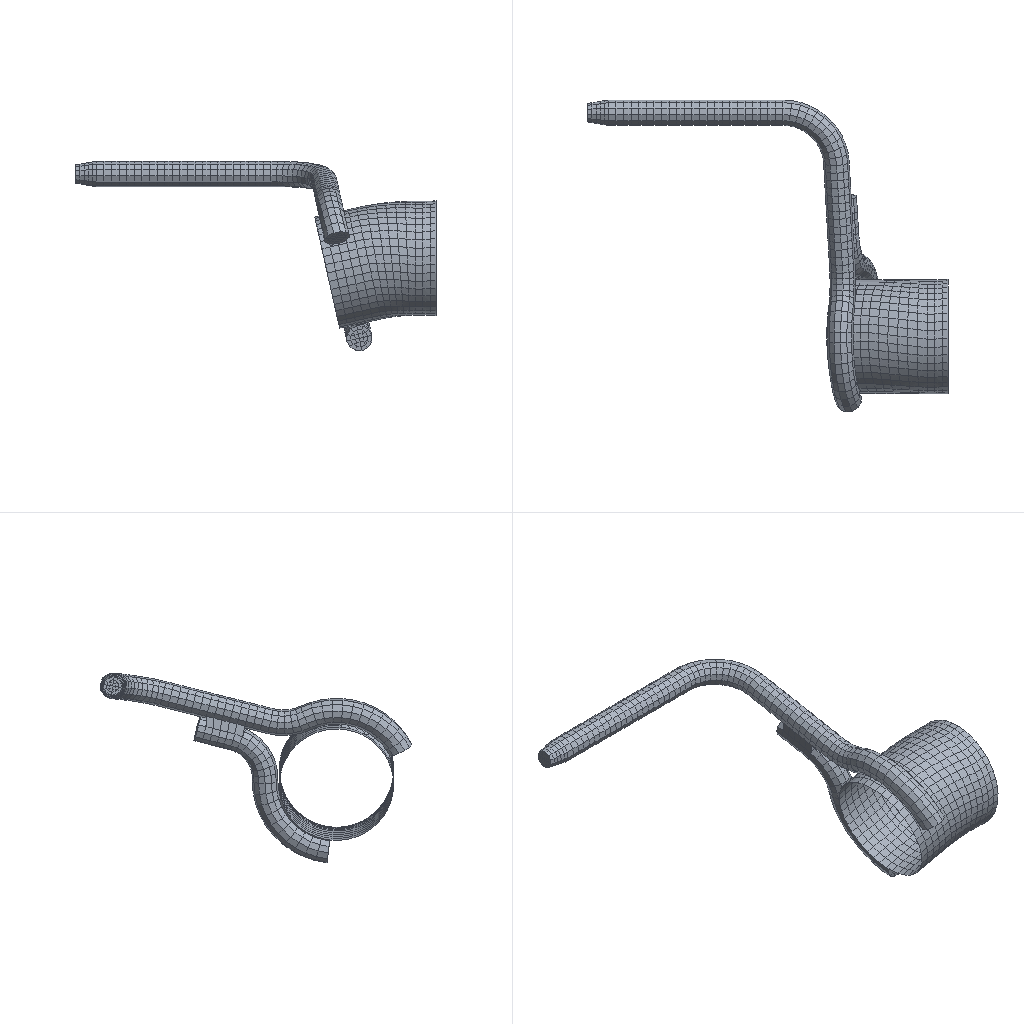Simulation study | nastran
Set-up summary:
category,name,step,type,value,unit,region
solver,nx_nastran
units,not stated in the deck,,not stated
analysis,deck,,modal,modal
analysis,solution,,SOL,103
load_step,SUBCASE 1,1,SUBCASE,SPC=None LOAD=None
mesh,nodes,,,3767
mesh,elements,,,633
element_type,CHEXA,,unverified,2232
element_type,CELAS1,,scalar,3
element_type,CPENTA,,unverified,372
element_type,CQUAD4,,shell,628
element_type,CTRIA3,,shell,2
load,load commands in deck,,count,0
bc,support commands in deck,,count,0
check,setup vs results,,match,"every grid point's frame and coordinates and every element id; grid points of CHEXA, CPENTA, CQUAD4, CTRIA3 elements"
Nastran input file, long lists of numbers shortened:
$$------------------------------------------------------------------------------$
$$                                                                              $
$$ NASTRAN Input Deck Generated by HyperMesh Version  :12.0.0.85
$$ Generated using HyperMesh-Nastran Template Version : 12.0
$$                                                                              $
$$   Template:  general                                                         $
$$                                                                              $
$$------------------------------------------------------------------------------$
$$------------------------------------------------------------------------------$
$$                      Executive Control Cards                                 $
$$------------------------------------------------------------------------------$
SOL 103
CEND
$$------------------------------------------------------------------------------$
$$                      Case Control Cards                                      $
$$------------------------------------------------------------------------------$
SET 2 = 1
$HMSET        2        1 "_PickedSet18"
$HMSETTYPE       2 "regular"
SET 3 = 2
$HMSET        3        1 "_PickedSet19"
$HMSETTYPE       3 "regular"
SET 4 = 7500,7527,7534,7541,7550,7554,
        7558,7559,7578,7582,7586,7587,
        7604,7613,7617,7621,7622,7642,
        7647,7648,7653,7654,7714,7721,
        7730,7734,7738,7739,7758,7762,
        7766,7767,7784,7793,7797,7801,
        7802,7822,7827,7828,7833,7834,
        283535,283558 THRU 283578,
        283749 THRU 283768
$HMSET        4        1 "_PickedSet6"
$HMSETTYPE       4 "regular"
SET 1 = 339780 THRU 339827,339872 THRU 339919,
        339946 THRU 339969,340010 THRU 340057,
        340102 THRU 340149,340167 THRU 340178,
        340208 THRU 340243,340277 THRU 340312,
        340337 THRU 340360,340374 THRU 340385,
        340397 THRU 340408,340420 THRU 340431,
        340443 THRU 340454,340475 THRU 340498
$HMSET        1        1 "_PickedSet17"
$HMSETTYPE       1 "regular"
$
$HMNAME LOADSTEP               1"Mode"
SUBCASE       1
  LABEL= Mode
  METHOD(STRUCTURE) =        1
  ANALYSIS = MODES
  DISPLACEMENT(SORT1,PHASE) = ALL
$$------------------------------------------------------------------------------$
$$                      Bulk Data Cards                                         $
$$------------------------------------------------------------------------------$
BEGIN BULK
PARAM,AUTOSPC,YES
PARAM,POST,-1
$$
$$  GRID Data
$$
GRID           1        382.471 104.72  112.379
GRID           2        382.529 104.106 132.44
$ (3765 more lines like these left out)
$$
$$  SPOINT Data
$$
$
$  CELAS1 Elements
$
CELAS1         3       9       1       3       2       3
CELAS1         2       8       1       2       2       2
CELAS1         1       7       1       1       2       1
$
$HMMOVE        6
$              3
$
$
$HMMOVE        7
$              2
$
$
$HMMOVE        8
$              1
$
$$
$$------------------------------------------------------------------------------$
$$             Group Definitions                                                $
$$------------------------------------------------------------------------------$
$$
$$ RBE2 Elements - Multiple dependent nodes
$$
RBE2      425190       1  123456  339780  339781  339782  339783  339784+
+         339785  339786  339787  339788  339789  339790  339791  339792+
+         339793  339794  339795  339796  339797  339798  339799  339800+
+         339801  339802  339803  339804  339805  339806  339807  339808+
+         339809  339810  339811  339812  339813  339814  339815  339816+
+         339817  339818  339819  339820  339821  339822  339823  339824+
+         339825  339826  339827  339872  339873  339874  339875  339876+
+         339877  339878  339879  339880  339881  339882  339883  339884+
+         339885  339886  339887  339888  339889  339890  339891  339892+
+         339893  339894  339895  339896  339897  339898  339899  339900+
+         339901  339902  339903  339904  339905  339906  339907  339908+
+         339909  339910  339911  339912  339913  339914  339915  339916+
+         339917  339918  339919  339946  339947  339948  339949  339950+
+         339951  339952  339953  339954  339955  339956  339957  339958+
+         339959  339960  339961  339962  339963  339964  339965  339966+
+         339967  339968  339969  340010  340011  340012  340013  340014+
+         340015  340016  340017  340018  340019  340020  340021  340022+
+         340023  340024  340025  340026  340027  340028  340029  340030+
+         340031  340032  340033  340034  340035  340036  340037  340038+
+         340039  340040  340041  340042  340043  340044  340045  340046+
+         340047  340048  340049  340050  340051  340052  340053  340054+
+         340055  340056  340057  340102  340103  340104  340105  340106+
+         340107  340108  340109  340110  340111  340112  340113  340114+
+         340115  340116  340117  340118  340119  340120  340121  340122+
+         340123  340124  340125  340126  340127  340128  340129  340130+
+         340131  340132  340133  340134  340135  340136  340137  340138+
+         340139  340140  340141  340142  340143  340144  340145  340146+
+         340147  340148  340149  340167  340168  340169  340170  340171+
+         340172  340173  340174  340175  340176  340177  340178  340208+
+         340209  340210  340211  340212  340213  340214  340215  340216+
+         340217  340218  340219  340220  340221  340222  340223  340224+
+         340225  340226  340227  340228  340229  340230  340231  340232+
+         340233  340234  340235  340236  340237  340238  340239  340240+
+         340241  340242  340243  340277  340278  340279  340280  340281+
+         340282  340283  340284  340285  340286  340287  340288  340289+
+         340290  340291  340292  340293  340294  340295  340296  340297+
+         340298  340299  340300  340301  340302  340303  340304  340305+
+         340306  340307  340308  340309  340310  340311  340312  340337+
+         340338  340339  340340  340341  340342  340343  340344  340345+
+         340346  340347  340348  340349  340350  340351  340352  340353+
+         340354  340355  340356  340357  340358  340359  340360  340374+
+         340375  340376  340377  340378  340379  340380  340381  340382+
+         340383  340384  340385  340397  340398  340399  340400  340401+
+         340402  340403  340404  340405  340406  340407  340408  340420+
+         340421  340422  340423  340424  340425  340426  340427  340428+
+         340429  340430  340431  340443  340444  340445  340446  340447+
+         340448  340449  340450  340451  340452  340453  340454  340475+
+         340476  340477  340478  340479  340480  340481  340482  340483+
+         340484  340485  340486  340487  340488  340489  340490  340491+
+         340492  340493  340494  340495  340496  340497  340498
$
$HMMOVE        2
$         425190
$
$$
$$  CTRIA3 Data
$$
CTRIA3    425153       6  338570  338568  320944
CTRIA3    425159       6  320941  338588  338589
$
$HMMOVE        4
$         425153  425159
$
$
$  CQUAD4 Elements
$
CQUAD4    425148       6  338353  320968  320970  338562
CQUAD4    425149       6  338562  320970  320925  338564
$ (626 more lines like these left out)
$
$HMMOVE        4
$         425148THRU      425152  425154THRU      425158  425160THRU      425189
$
$
$HMMOVE        5
$           7287THRU        7288    7296    7299THRU        7300    7327THRU
$           7328    7336    7339THRU        7340    7367THRU        7368    7376
$           7379THRU        7380    7412    7415THRU        7416    7424    7427
$       THRU        7428    7455THRU        7456    7464    7467THRU        7468
$           7495THRU        7496    7504    7507THRU        7508    7535THRU
$           7536    7544    7547THRU        7548    7580    7583THRU        7584
$           7592    7595THRU        7596    9681THRU       10016  302613  302615
$         302617  302619  302621  302623  302625  302627  302629  302631  302633
$         302635  302637  302639  302641  302643  302645  302647  302649  302651
$         302653  302781  302783  302785  302787  302789  302791  302793  302795
$         302797  302799  302801  302803  302805  302807  302809  302811  302813
$         302815  302817  302819  302821  343457THRU      343624
$
$
$  CHEXA Elements: First Order
$
CHEXA     367608       4  338326  338334  338328  338327  338357  338360+
+         338359  338358
CHEXA     367609       4  338357  338360  338359  338358  338361  338364+
+         338363  338362
$ (4460 more lines like these left out)
$
$HMMOVE        3
$         367608THRU      367655  367668THRU      367691  367704THRU      367775
$         367788THRU      367895  367908THRU      367958  367964THRU      368003
$         368009THRU      368058  368064THRU      368073  368079THRU      368083
$         368348THRU      368371  368376THRU      368399  368404THRU      368427
$         368432THRU      368455  368460THRU      368483  368488THRU      368511
$         368516THRU      368539  368544THRU      368567  368572THRU      368595
$         368600THRU      368623  368628THRU      368651  368656THRU      368679
$         368684THRU      368707  368712THRU      368735  369004THRU      369267
$         369624THRU      370152  370245THRU      370267  370900THRU      370954
$         370975THRU      371039  371080THRU      371104  371110THRU      371114
$         371120THRU      371174  371180THRU      371184  371190THRU      371219
$         372060THRU      372251  373196THRU      373435
$
$$
$$------------------------------------------------------------------------------$
$$    HyperMesh name information for generic property collectors                $
$$------------------------------------------------------------------------------$
$$
$$------------------------------------------------------------------------------$
$$    Property Definition for 1-D Elements                                      $
$$------------------------------------------------------------------------------$
$
$  CPENTA Elements 6-noded
$
CPENTA    367656       4  338335  338334  338333  338405  338360  338408
CPENTA    367657       4  338405  338360  338408  338409  338364  338412
$ (370 more lines like these left out)
$
$HMMOVE        3
$         367656THRU      367667  367692THRU      367703  367776THRU      367787
$         367896THRU      367907  367959THRU      367963  368004THRU      368008
$ (49 more lines like these left out)
PSHELL         5       11.0            1               1
$
$HMNAME PROP                   6"HANJIE" 4
$HWCOLOR PROP                  6       7
PSHELL         6       13.0            1               1
$$
$$  PSOLID Data
$
$HMNAME PROP                   4"FUJIAN-3D" 5
$HWCOLOR PROP                  4       8
PSOLID         4       1
$$
$$  PELAS Data
$
$HMNAME PROP                   7"Springs/Dashpots-1-spring" 2
$HWCOLOR PROP                  7       3
PELAS          712.0    0.0     0.0
$
$HMNAME PROP                   8"Springs/Dashpots-1-Copy-spring" 2
$HWCOLOR PROP                  8       4
PELAS          88.0     0.0     0.0
$
$HMNAME PROP                   9"Springs/Dashpots-1-Copy-Copy-spring" 2
$HWCOLOR PROP                  9       5
PELAS          910.0    0.0     0.0
$$--------------------------------------------------------------
$$ HYPERMESH TAGS
$$--------------------------------------------------------------
$$BEGIN TAGS
$$END TAGS
$$
$$  MAT1 Data
$
$HMNAME MAT                    1"sus409" "MAT1"
$HWCOLOR MAT                   1       3
MAT1           1209000.0        0.33    7.71-9
$$
$$
$$
$$------------------------------------------------------------------------------$
$$     HyperMesh name information for generic materials                         $
$$------------------------------------------------------------------------------$
$$
$$------------------------------------------------------------------------------$
$$                      Material Definition Cards                               $
$$------------------------------------------------------------------------------$
$$
$$------------------------------------------------------------------------------$
$$        Loads and Boundary Conditions                                         $
$$------------------------------------------------------------------------------$
$$
$$HyperMesh name and color information for generic loadcollectors
$$
$$
$$
$$
$$
$$
$$
$$
$$  EIGRL cards
$$
$HMNAME LOADCOL                1"Eigrl"
$HWCOLOR LOADCOL               1      11
EIGRL          1        2000.0                                      MASS
$
ENDDATA
Results summary:
result,analysis,,,modal
result,primary field,,,eigenvectors